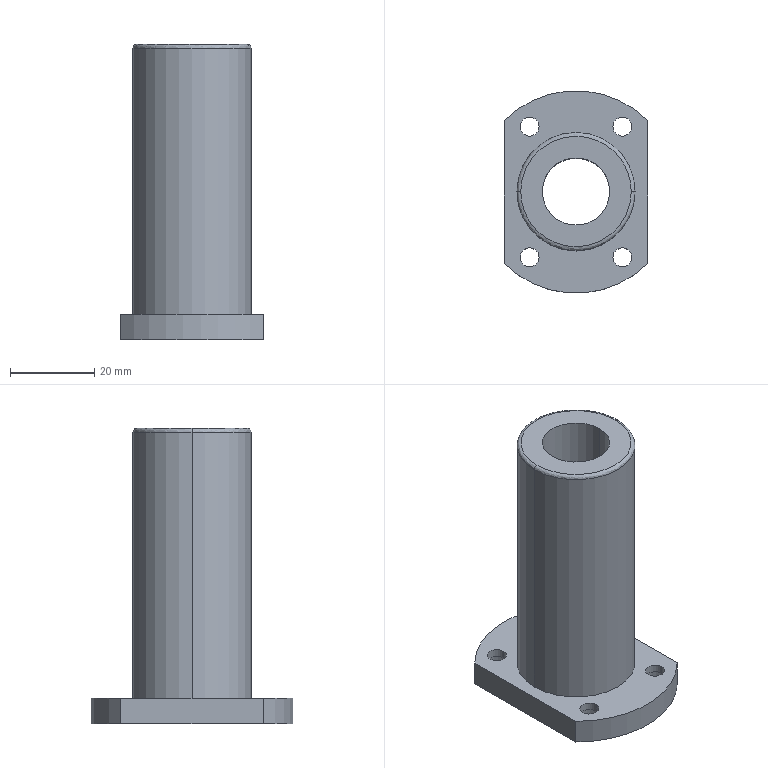Part | SolidWorks | features BaseBody 1 | 1 solid | 33 faces | box 34 x 48 x 70 mm | volume 33372 mm3 | cylinder 22 | plane 9 | spline 2 | commonest cylinder face diameters 4.5 x8 7.5 x8 16 x2 28 x2 48 x2
STEP:
#1=CARTESIAN_POINT('',(14.,0.,69.1));
#2=VERTEX_POINT('',#1);
#3=CARTESIAN_POINT('',(-14.,0.,69.1));
#4=VERTEX_POINT('',#3);
#5=CARTESIAN_POINT('',(0.,0.,69.1));
#6=DIRECTION('',(0.,0.,-1.));
#7=DIRECTION('',(-1.,0.,0.));
#8=AXIS2_PLACEMENT_3D('',#5,#6,#7);
#9=CIRCLE('',#8,14.);
#10=EDGE_CURVE('',#2,#4,#9,.T.);
#11=ORIENTED_EDGE('',*,*,#10,.F.);
#12=CARTESIAN_POINT('',(13.1,0.,70.));
#13=VERTEX_POINT('',#12);
#14=CARTESIAN_POINT('',(13.1,0.,69.1));
#15=DIRECTION('',(0.,-1.,0.));
#16=DIRECTION('',(1.,0.,0.));
#17=AXIS2_PLACEMENT_3D('',#14,#15,#16);
#18=CIRCLE('',#17,0.9);
#19=EDGE_CURVE('',#2,#13,#18,.T.);
#20=ORIENTED_EDGE('',*,*,#19,.T.);
#21=CARTESIAN_POINT('',(-13.1,0.,70.));
#22=VERTEX_POINT('',#21);
#23=CARTESIAN_POINT('',(13.1,0.,70.));
#24=CARTESIAN_POINT('',(13.1,-26.2,70.));
#25=CARTESIAN_POINT('',(-13.1,-26.2,70.));
#26=CARTESIAN_POINT('',(-13.1,0.,70.));
#27=(BOUNDED_CURVE()B_SPLINE_CURVE(3,(#23,#24,#25,#26),.UNSPECIFIED.,.F.,.F.)B_SPLINE_CURVE_WITH_KNOTS((4,4),(0.5,1.),.UNSPECIFIED.)CURVE()GEOMETRIC_REPRESENTATION_ITEM()RATIONAL_B_SPLINE_CURVE((1.,0.3333,0.3333,1.))REPRESENTATION_ITEM(''));
#28=EDGE_CURVE('',#13,#22,#27,.T.);
#29=ORIENTED_EDGE('',*,*,#28,.T.);
#30=CARTESIAN_POINT('',(-13.1,0.,69.1));
#31=DIRECTION('',(0.,1.,0.));
#32=DIRECTION('',(-1.,0.,0.));
#33=AXIS2_PLACEMENT_3D('',#30,#31,#32);
#34=CIRCLE('',#33,0.9);
#35=EDGE_CURVE('',#4,#22,#34,.T.);
#36=ORIENTED_EDGE('',*,*,#35,.F.);
#37=EDGE_LOOP('',(#11,#20,#29,#36));
#38=FACE_OUTER_BOUND('',#37,.T.);
#39=CARTESIAN_POINT('',(14.,0.,69.1));
#40=CARTESIAN_POINT('',(14.,-28.,69.1));
#41=CARTESIAN_POINT('',(-14.,-28.,69.1));
#42=CARTESIAN_POINT('',(-14.,0.,69.1));
#43=CARTESIAN_POINT('',(14.,0.,69.627));
#44=CARTESIAN_POINT('',(14.,-28.,69.627));
#45=CARTESIAN_POINT('',(-14.,-28.,69.627));
#46=CARTESIAN_POINT('',(-14.,0.,69.627));
#47=CARTESIAN_POINT('',(13.627,0.,70.));
#48=CARTESIAN_POINT('',(13.627,-27.254,70.));
#49=CARTESIAN_POINT('',(-13.627,-27.254,70.));
#50=CARTESIAN_POINT('',(-13.627,0.,70.));
#51=CARTESIAN_POINT('',(13.1,0.,70.));
#52=CARTESIAN_POINT('',(13.1,-26.2,70.));
#53=CARTESIAN_POINT('',(-13.1,-26.2,70.));
#54=CARTESIAN_POINT('',(-13.1,0.,70.));
#55=(BOUNDED_SURFACE()B_SPLINE_SURFACE(3,3,((#39,#40,#41,#42),(#43,#44,#45,#46),(#47,#48,#49,#50),(#51,#52,#53,#54)),.UNSPECIFIED.,.F.,.F.,.F.)B_SPLINE_SURFACE_WITH_KNOTS((4,4),(4,4),(0.,1.),(0.,1.),.UNSPECIFIED.)GEOMETRIC_REPRESENTATION_ITEM()RATIONAL_B_SPLINE_SURFACE(((1.,0.3333,0.3333,1.),(0.8047,0.2682,0.2682,0.8047),(0.8047,0.2682,0.2682,0.8047),(1.,0.3333,0.3333,1.)))REPRESENTATION_ITEM('')SURFACE());
#56=ADVANCED_FACE('',(#38),#55,.T.);
#57=CARTESIAN_POINT('',(0.,0.,69.1));
#58=DIRECTION('',(0.,0.,-1.));
#59=DIRECTION('',(-1.,0.,0.));
#60=AXIS2_PLACEMENT_3D('',#57,#58,#59);
#61=CIRCLE('',#60,14.);
#62=EDGE_CURVE('',#4,#2,#61,.T.);
#63=ORIENTED_EDGE('',*,*,#62,.T.);
#64=CARTESIAN_POINT('',(14.,0.,6.));
#65=VERTEX_POINT('',#64);
#66=CARTESIAN_POINT('',(14.,0.,0.));
#67=DIRECTION('',(0.,0.,-1.));
#68=VECTOR('',#67,1000.);
#69=LINE('',#66,#68);
#70=EDGE_CURVE('',#2,#65,#69,.T.);
#71=ORIENTED_EDGE('',*,*,#70,.T.);
#72=CARTESIAN_POINT('',(-14.,0.,6.));
#73=VERTEX_POINT('',#72);
#74=CARTESIAN_POINT('',(0.,0.,6.));
#75=DIRECTION('',(0.,0.,1.));
#76=DIRECTION('',(-1.,0.,0.));
#77=AXIS2_PLACEMENT_3D('',#74,#75,#76);
#78=CIRCLE('',#77,14.);
#79=EDGE_CURVE('',#65,#73,#78,.T.);
#80=ORIENTED_EDGE('',*,*,#79,.T.);
#81=CARTESIAN_POINT('',(-14.,0.,0.));
#82=DIRECTION('',(0.,0.,-1.));
#83=VECTOR('',#82,1000.);
#84=LINE('',#81,#83);
#85=EDGE_CURVE('',#4,#73,#84,.T.);
#86=ORIENTED_EDGE('',*,*,#85,.F.);
#87=EDGE_LOOP('',(#63,#71,#80,#86));
#88=FACE_OUTER_BOUND('',#87,.T.);
#89=CARTESIAN_POINT('',(0.,0.,0.));
#90=DIRECTION('',(0.,0.,-1.));
#91=DIRECTION('',(-1.,0.,0.));
#92=AXIS2_PLACEMENT_3D('',#89,#90,#91);
#93=CYLINDRICAL_SURFACE('',#92,14.);
#94=ADVANCED_FACE('',(#88),#93,.T.);
#95=CARTESIAN_POINT('',(-8.75,15.5,6.));
#96=VERTEX_POINT('',#95);
#97=CARTESIAN_POINT('',(-13.25,15.5,6.));
#98=VERTEX_POINT('',#97);
#99=CARTESIAN_POINT('',(-11.,15.5,6.));
#100=DIRECTION('',(0.,0.,-1.));
#101=DIRECTION('',(-1.,0.,0.));
#102=AXIS2_PLACEMENT_3D('',#99,#100,#101);
#103=CIRCLE('',#102,2.25);
#104=EDGE_CURVE('',#96,#98,#103,.T.);
#105=ORIENTED_EDGE('',*,*,#104,.F.);
#106=CARTESIAN_POINT('',(-8.75,15.5,4.1));
#107=VERTEX_POINT('',#106);
#108=CARTESIAN_POINT('',(-8.75,15.5,0.));
#109=DIRECTION('',(0.,0.,-1.));
#110=VECTOR('',#109,1000.);
#111=LINE('',#108,#110);
#112=EDGE_CURVE('',#96,#107,#111,.T.);
#113=ORIENTED_EDGE('',*,*,#112,.T.);
#114=CARTESIAN_POINT('',(-13.25,15.5,4.1));
#115=VERTEX_POINT('',#114);
#116=CARTESIAN_POINT('',(-11.,15.5,4.1));
#117=DIRECTION('',(0.,0.,1.));
#118=DIRECTION('',(-1.,0.,0.));
#119=AXIS2_PLACEMENT_3D('',#116,#117,#118);
#120=CIRCLE('',#119,2.25);
#121=EDGE_CURVE('',#115,#107,#120,.T.);
#122=ORIENTED_EDGE('',*,*,#121,.F.);
#123=CARTESIAN_POINT('',(-13.25,15.5,0.));
#124=DIRECTION('',(0.,0.,-1.));
#125=VECTOR('',#124,1000.);
#126=LINE('',#123,#125);
#127=EDGE_CURVE('',#98,#115,#126,.T.);
#128=ORIENTED_EDGE('',*,*,#127,.F.);
#129=EDGE_LOOP('',(#105,#113,#122,#128));
#130=FACE_OUTER_BOUND('',#129,.T.);
#131=CARTESIAN_POINT('',(-11.,15.5,0.));
#132=DIRECTION('',(0.,0.,-1.));
#133=DIRECTION('',(-1.,0.,0.));
#134=AXIS2_PLACEMENT_3D('',#131,#132,#133);
#135=CYLINDRICAL_SURFACE('',#134,2.25);
#136=ADVANCED_FACE('',(#130),#135,.F.);
#137=CARTESIAN_POINT('',(-13.25,-15.5,4.1));
#138=VERTEX_POINT('',#137);
#139=CARTESIAN_POINT('',(-8.75,-15.5,4.1));
#140=VERTEX_POINT('',#139);
#141=CARTESIAN_POINT('',(-11.,-15.5,4.1));
#142=DIRECTION('',(0.,0.,1.));
#143=DIRECTION('',(1.,0.,0.));
#144=AXIS2_PLACEMENT_3D('',#141,#142,#143);
#145=CIRCLE('',#144,2.25);
#146=EDGE_CURVE('',#138,#140,#145,.T.);
#147=ORIENTED_EDGE('',*,*,#146,.F.);
#148=CARTESIAN_POINT('',(-13.25,-15.5,6.));
#149=VERTEX_POINT('',#148);
#150=CARTESIAN_POINT('',(-13.25,-15.5,6.));
#151=DIRECTION('',(0.,0.,1.));
#152=VECTOR('',#151,1000.);
#153=LINE('',#150,#152);
#154=EDGE_CURVE('',#138,#149,#153,.T.);
#155=ORIENTED_EDGE('',*,*,#154,.T.);
#156=CARTESIAN_POINT('',(-8.75,-15.5,6.));
#157=VERTEX_POINT('',#156);
#158=CARTESIAN_POINT('',(-11.,-15.5,6.));
#159=DIRECTION('',(0.,0.,-1.));
#160=DIRECTION('',(1.,0.,0.));
#161=AXIS2_PLACEMENT_3D('',#158,#159,#160);
#162=CIRCLE('',#161,2.25);
#163=EDGE_CURVE('',#157,#149,#162,.T.);
#164=ORIENTED_EDGE('',*,*,#163,.F.);
#165=CARTESIAN_POINT('',(-8.75,-15.5,6.));
#166=DIRECTION('',(0.,0.,1.));
#167=VECTOR('',#166,1000.);
#168=LINE('',#165,#167);
#169=EDGE_CURVE('',#140,#157,#168,.T.);
#170=ORIENTED_EDGE('',*,*,#169,.F.);
#171=EDGE_LOOP('',(#147,#155,#164,#170));
#172=FACE_OUTER_BOUND('',#171,.T.);
#173=CARTESIAN_POINT('',(-11.,-15.5,6.));
#174=DIRECTION('',(0.,0.,1.));
#175=DIRECTION('',(1.,0.,0.));
#176=AXIS2_PLACEMENT_3D('',#173,#174,#175);
#177=CYLINDRICAL_SURFACE('',#176,2.25);
#178=ADVANCED_FACE('',(#172),#177,.F.);
#179=CARTESIAN_POINT('',(13.25,15.5,6.));
#180=VERTEX_POINT('',#179);
#181=CARTESIAN_POINT('',(8.75,15.5,6.));
#182=VERTEX_POINT('',#181);
#183=CARTESIAN_POINT('',(11.,15.5,6.));
#184=DIRECTION('',(0.,0.,-1.));
#185=DIRECTION('',(-1.,0.,0.));
#186=AXIS2_PLACEMENT_3D('',#183,#184,#185);
#187=CIRCLE('',#186,2.25);
#188=EDGE_CURVE('',#180,#182,#187,.T.);
#189=ORIENTED_EDGE('',*,*,#188,.F.);
#190=CARTESIAN_POINT('',(13.25,15.5,4.1));
#191=VERTEX_POINT('',#190);
#192=CARTESIAN_POINT('',(13.25,15.5,0.));
#193=DIRECTION('',(0.,0.,-1.));
#194=VECTOR('',#193,1000.);
#195=LINE('',#192,#194);
#196=EDGE_CURVE('',#180,#191,#195,.T.);
#197=ORIENTED_EDGE('',*,*,#196,.T.);
#198=CARTESIAN_POINT('',(8.75,15.5,4.1));
#199=VERTEX_POINT('',#198);
#200=CARTESIAN_POINT('',(11.,15.5,4.1));
#201=DIRECTION('',(0.,0.,1.));
#202=DIRECTION('',(-1.,0.,0.));
#203=AXIS2_PLACEMENT_3D('',#200,#201,#202);
#204=CIRCLE('',#203,2.25);
#205=EDGE_CURVE('',#199,#191,#204,.T.);
#206=ORIENTED_EDGE('',*,*,#205,.F.);
#207=CARTESIAN_POINT('',(8.75,15.5,0.));
#208=DIRECTION('',(0.,0.,-1.));
#209=VECTOR('',#208,1000.);
#210=LINE('',#207,#209);
#211=EDGE_CURVE('',#182,#199,#210,.T.);
#212=ORIENTED_EDGE('',*,*,#211,.F.);
#213=EDGE_LOOP('',(#189,#197,#206,#212));
#214=FACE_OUTER_BOUND('',#213,.T.);
#215=CARTESIAN_POINT('',(11.,15.5,0.));
#216=DIRECTION('',(0.,0.,-1.));
#217=DIRECTION('',(-1.,0.,0.));
#218=AXIS2_PLACEMENT_3D('',#215,#216,#217);
#219=CYLINDRICAL_SURFACE('',#218,2.25);
#220=ADVANCED_FACE('',(#214),#219,.F.);
#221=CARTESIAN_POINT('',(8.75,-15.5,4.1));
#222=VERTEX_POINT('',#221);
#223=CARTESIAN_POINT('',(13.25,-15.5,4.1));
#224=VERTEX_POINT('',#223);
#225=CARTESIAN_POINT('',(11.,-15.5,4.1));
#226=DIRECTION('',(0.,0.,1.));
#227=DIRECTION('',(1.,0.,0.));
#228=AXIS2_PLACEMENT_3D('',#225,#226,#227);
#229=CIRCLE('',#228,2.25);
#230=EDGE_CURVE('',#222,#224,#229,.T.);
#231=ORIENTED_EDGE('',*,*,#230,.F.);
#232=CARTESIAN_POINT('',(8.75,-15.5,6.));
#233=VERTEX_POINT('',#232);
#234=CARTESIAN_POINT('',(8.75,-15.5,6.));
#235=DIRECTION('',(0.,0.,1.));
#236=VECTOR('',#235,1000.);
#237=LINE('',#234,#236);
#238=EDGE_CURVE('',#222,#233,#237,.T.);
#239=ORIENTED_EDGE('',*,*,#238,.T.);
#240=CARTESIAN_POINT('',(13.25,-15.5,6.));
#241=VERTEX_POINT('',#240);
#242=CARTESIAN_POINT('',(11.,-15.5,6.));
#243=DIRECTION('',(0.,0.,-1.));
#244=DIRECTION('',(1.,0.,0.));
#245=AXIS2_PLACEMENT_3D('',#242,#243,#244);
#246=CIRCLE('',#245,2.25);
#247=EDGE_CURVE('',#241,#233,#246,.T.);
#248=ORIENTED_EDGE('',*,*,#247,.F.);
#249=CARTESIAN_POINT('',(13.25,-15.5,6.));
#250=DIRECTION('',(0.,0.,1.));
#251=VECTOR('',#250,1000.);
#252=LINE('',#249,#251);
#253=EDGE_CURVE('',#224,#241,#252,.T.);
#254=ORIENTED_EDGE('',*,*,#253,.F.);
#255=EDGE_LOOP('',(#231,#239,#248,#254));
#256=FACE_OUTER_BOUND('',#255,.T.);
#257=CARTESIAN_POINT('',(11.,-15.5,6.));
#258=DIRECTION('',(0.,0.,1.));
#259=DIRECTION('',(1.,0.,0.));
#260=AXIS2_PLACEMENT_3D('',#257,#258,#259);
#261=CYLINDRICAL_SURFACE('',#260,2.25);
#262=ADVANCED_FACE('',(#256),#261,.F.);
#263=CARTESIAN_POINT('',(8.,0.,70.));
#264=VERTEX_POINT('',#263);
#265=CARTESIAN_POINT('',(-8.,0.,70.));
#266=VERTEX_POINT('',#265);
#267=CARTESIAN_POINT('',(0.,0.,70.));
#268=DIRECTION('',(0.,0.,-1.));
#269=DIRECTION('',(-1.,0.,0.));
#270=AXIS2_PLACEMENT_3D('',#267,#268,#269);
#271=CIRCLE('',#270,8.);
#272=EDGE_CURVE('',#264,#266,#271,.T.);
#273=ORIENTED_EDGE('',*,*,#272,.F.);
#274=CARTESIAN_POINT('',(8.,0.,0.));
#275=VERTEX_POINT('',#274);
#276=CARTESIAN_POINT('',(8.,0.,0.));
#277=DIRECTION('',(0.,0.,-1.));
#278=VECTOR('',#277,1000.);
#279=LINE('',#276,#278);
#280=EDGE_CURVE('',#264,#275,#279,.T.);
#281=ORIENTED_EDGE('',*,*,#280,.T.);
#282=CARTESIAN_POINT('',(-8.,0.,0.));
#283=VERTEX_POINT('',#282);
#284=CARTESIAN_POINT('',(0.,0.,0.));
#285=DIRECTION('',(0.,0.,1.));
#286=DIRECTION('',(-1.,0.,0.));
#287=AXIS2_PLACEMENT_3D('',#284,#285,#286);
#288=CIRCLE('',#287,8.);
#289=EDGE_CURVE('',#283,#275,#288,.T.);
#290=ORIENTED_EDGE('',*,*,#289,.F.);
#291=CARTESIAN_POINT('',(-8.,0.,0.));
#292=DIRECTION('',(0.,0.,-1.));
#293=VECTOR('',#292,1000.);
#294=LINE('',#291,#293);
#295=EDGE_CURVE('',#266,#283,#294,.T.);
#296=ORIENTED_EDGE('',*,*,#295,.F.);
#297=EDGE_LOOP('',(#273,#281,#290,#296));
#298=FACE_OUTER_BOUND('',#297,.T.);
#299=CARTESIAN_POINT('',(0.,0.,0.));
#300=DIRECTION('',(0.,0.,-1.));
#301=DIRECTION('',(-1.,0.,0.));
#302=AXIS2_PLACEMENT_3D('',#299,#300,#301);
#303=CYLINDRICAL_SURFACE('',#302,8.);
#304=ADVANCED_FACE('',(#298),#303,.F.);
#305=CARTESIAN_POINT('',(-7.25,15.5,4.1));
#306=VERTEX_POINT('',#305);
#307=CARTESIAN_POINT('',(-14.75,15.5,4.1));
#308=VERTEX_POINT('',#307);
#309=CARTESIAN_POINT('',(-11.,15.5,4.1));
#310=DIRECTION('',(0.,0.,-1.));
#311=DIRECTION('',(-1.,0.,0.));
#312=AXIS2_PLACEMENT_3D('',#309,#310,#311);
#313=CIRCLE('',#312,3.75);
#314=EDGE_CURVE('',#306,#308,#313,.T.);
#315=ORIENTED_EDGE('',*,*,#314,.F.);
#316=CARTESIAN_POINT('',(-7.25,15.5,0.));
#317=VERTEX_POINT('',#316);
#318=CARTESIAN_POINT('',(-7.25,15.5,0.));
#319=DIRECTION('',(0.,0.,-1.));
#320=VECTOR('',#319,1000.);
#321=LINE('',#318,#320);
#322=EDGE_CURVE('',#306,#317,#321,.T.);
#323=ORIENTED_EDGE('',*,*,#322,.T.);
#324=CARTESIAN_POINT('',(-14.75,15.5,0.));
#325=VERTEX_POINT('',#324);
#326=CARTESIAN_POINT('',(-11.,15.5,0.));
#327=DIRECTION('',(0.,0.,1.));
#328=DIRECTION('',(-1.,0.,0.));
#329=AXIS2_PLACEMENT_3D('',#326,#327,#328);
#330=CIRCLE('',#329,3.75);
#331=EDGE_CURVE('',#325,#317,#330,.T.);
#332=ORIENTED_EDGE('',*,*,#331,.F.);
#333=CARTESIAN_POINT('',(-14.75,15.5,0.));
#334=DIRECTION('',(0.,0.,-1.));
#335=VECTOR('',#334,1000.);
#336=LINE('',#333,#335);
#337=EDGE_CURVE('',#308,#325,#336,.T.);
#338=ORIENTED_EDGE('',*,*,#337,.F.);
#339=EDGE_LOOP('',(#315,#323,#332,#338));
#340=FACE_OUTER_BOUND('',#339,.T.);
#341=CARTESIAN_POINT('',(-11.,15.5,0.));
#342=DIRECTION('',(0.,0.,-1.));
#343=DIRECTION('',(-1.,0.,0.));
#344=AXIS2_PLACEMENT_3D('',#341,#342,#343);
#345=CYLINDRICAL_SURFACE('',#344,3.75);
#346=ADVANCED_FACE('',(#340),#345,.F.);
#347=CARTESIAN_POINT('',(-14.75,-15.5,0.));
#348=VERTEX_POINT('',#347);
#349=CARTESIAN_POINT('',(-7.25,-15.5,0.));
#350=VERTEX_POINT('',#349);
#351=CARTESIAN_POINT('',(-11.,-15.5,0.));
#352=DIRECTION('',(0.,0.,1.));
#353=DIRECTION('',(1.,0.,0.));
#354=AXIS2_PLACEMENT_3D('',#351,#352,#353);
#355=CIRCLE('',#354,3.75);
#356=EDGE_CURVE('',#348,#350,#355,.T.);
#357=ORIENTED_EDGE('',*,*,#356,.F.);
#358=CARTESIAN_POINT('',(-14.75,-15.5,4.1));
#359=VERTEX_POINT('',#358);
#360=CARTESIAN_POINT('',(-14.75,-15.5,6.));
#361=DIRECTION('',(0.,0.,1.));
#362=VECTOR('',#361,1000.);
#363=LINE('',#360,#362);
#364=EDGE_CURVE('',#348,#359,#363,.T.);
#365=ORIENTED_EDGE('',*,*,#364,.T.);
#366=CARTESIAN_POINT('',(-7.25,-15.5,4.1));
#367=VERTEX_POINT('',#366);
#368=CARTESIAN_POINT('',(-11.,-15.5,4.1));
#369=DIRECTION('',(0.,0.,-1.));
#370=DIRECTION('',(1.,0.,0.));
#371=AXIS2_PLACEMENT_3D('',#368,#369,#370);
#372=CIRCLE('',#371,3.75);
#373=EDGE_CURVE('',#367,#359,#372,.T.);
#374=ORIENTED_EDGE('',*,*,#373,.F.);
#375=CARTESIAN_POINT('',(-7.25,-15.5,6.));
#376=DIRECTION('',(0.,0.,1.));
#377=VECTOR('',#376,1000.);
#378=LINE('',#375,#377);
#379=EDGE_CURVE('',#350,#367,#378,.T.);
#380=ORIENTED_EDGE('',*,*,#379,.F.);
#381=EDGE_LOOP('',(#357,#365,#374,#380));
#382=FACE_OUTER_BOUND('',#381,.T.);
#383=CARTESIAN_POINT('',(-11.,-15.5,6.));
#384=DIRECTION('',(0.,0.,1.));
#385=DIRECTION('',(1.,0.,0.));
#386=AXIS2_PLACEMENT_3D('',#383,#384,#385);
#387=CYLINDRICAL_SURFACE('',#386,3.75);
#388=ADVANCED_FACE('',(#382),#387,.F.);
#389=CARTESIAN_POINT('',(14.75,15.5,4.1));
#390=VERTEX_POINT('',#389);
#391=CARTESIAN_POINT('',(7.25,15.5,4.1));
#392=VERTEX_POINT('',#391);
#393=CARTESIAN_POINT('',(11.,15.5,4.1));
#394=DIRECTION('',(0.,0.,-1.));
#395=DIRECTION('',(-1.,0.,0.));
#396=AXIS2_PLACEMENT_3D('',#393,#394,#395);
#397=CIRCLE('',#396,3.75);
#398=EDGE_CURVE('',#390,#392,#397,.T.);
#399=ORIENTED_EDGE('',*,*,#398,.F.);
#400=CARTESIAN_POINT('',(14.75,15.5,0.));
#401=VERTEX_POINT('',#400);
#402=CARTESIAN_POINT('',(14.75,15.5,0.));
#403=DIRECTION('',(0.,0.,-1.));
#404=VECTOR('',#403,1000.);
#405=LINE('',#402,#404);
#406=EDGE_CURVE('',#390,#401,#405,.T.);
#407=ORIENTED_EDGE('',*,*,#406,.T.);
#408=CARTESIAN_POINT('',(7.25,15.5,0.));
#409=VERTEX_POINT('',#408);
#410=CARTESIAN_POINT('',(11.,15.5,0.));
#411=DIRECTION('',(0.,0.,1.));
#412=DIRECTION('',(-1.,0.,0.));
#413=AXIS2_PLACEMENT_3D('',#410,#411,#412);
#414=CIRCLE('',#413,3.75);
#415=EDGE_CURVE('',#409,#401,#414,.T.);
#416=ORIENTED_EDGE('',*,*,#415,.F.);
#417=CARTESIAN_POINT('',(7.25,15.5,0.));
#418=DIRECTION('',(0.,0.,-1.));
#419=VECTOR('',#418,1000.);
#420=LINE('',#417,#419);
#421=EDGE_CURVE('',#392,#409,#420,.T.);
#422=ORIENTED_EDGE('',*,*,#421,.F.);
#423=EDGE_LOOP('',(#399,#407,#416,#422));
#424=FACE_OUTER_BOUND('',#423,.T.);
#425=CARTESIAN_POINT('',(11.,15.5,0.));
#426=DIRECTION('',(0.,0.,-1.));
#427=DIRECTION('',(-1.,0.,0.));
#428=AXIS2_PLACEMENT_3D('',#425,#426,#427);
#429=CYLINDRICAL_SURFACE('',#428,3.75);
#430=ADVANCED_FACE('',(#424),#429,.F.);
#431=CARTESIAN_POINT('',(7.25,-15.5,0.));
#432=VERTEX_POINT('',#431);
#433=CARTESIAN_POINT('',(14.75,-15.5,0.));
#434=VERTEX_POINT('',#433);
#435=CARTESIAN_POINT('',(11.,-15.5,0.));
#436=DIRECTION('',(0.,0.,1.));
#437=DIRECTION('',(1.,0.,0.));
#438=AXIS2_PLACEMENT_3D('',#435,#436,#437);
#439=CIRCLE('',#438,3.75);
#440=EDGE_CURVE('',#432,#434,#439,.T.);
#441=ORIENTED_EDGE('',*,*,#440,.F.);
#442=CARTESIAN_POINT('',(7.25,-15.5,4.1));
#443=VERTEX_POINT('',#442);
#444=CARTESIAN_POINT('',(7.25,-15.5,6.));
#445=DIRECTION('',(0.,0.,1.));
#446=VECTOR('',#445,1000.);
#447=LINE('',#444,#446);
#448=EDGE_CURVE('',#432,#443,#447,.T.);
#449=ORIENTED_EDGE('',*,*,#448,.T.);
#450=CARTESIAN_POINT('',(14.75,-15.5,4.1));
#451=VERTEX_POINT('',#450);
#452=CARTESIAN_POINT('',(11.,-15.5,4.1));
#453=DIRECTION('',(0.,0.,-1.));
#454=DIRECTION('',(1.,0.,0.));
#455=AXIS2_PLACEMENT_3D('',#452,#453,#454);
#456=CIRCLE('',#455,3.75);
#457=EDGE_CURVE('',#451,#443,#456,.T.);
#458=ORIENTED_EDGE('',*,*,#457,.F.);
#459=CARTESIAN_POINT('',(14.75,-15.5,6.));
#460=DIRECTION('',(0.,0.,1.));
#461=VECTOR('',#460,1000.);
#462=LINE('',#459,#461);
#463=EDGE_CURVE('',#434,#451,#462,.T.);
#464=ORIENTED_EDGE('',*,*,#463,.F.);
#465=EDGE_LOOP('',(#441,#449,#458,#464));
#466=FACE_OUTER_BOUND('',#465,.T.);
#467=CARTESIAN_POINT('',(11.,-15.5,6.));
#468=DIRECTION('',(0.,0.,1.));
#469=DIRECTION('',(1.,0.,0.));
#470=AXIS2_PLACEMENT_3D('',#467,#468,#469);
#471=CYLINDRICAL_SURFACE('',#470,3.75);
#472=ADVANCED_FACE('',(#466),#471,.F.);
#473=ORIENTED_EDGE('',*,*,#70,.F.);
#474=ORIENTED_EDGE('',*,*,#10,.T.);
#475=ORIENTED_EDGE('',*,*,#85,.T.);
#476=CARTESIAN_POINT('',(0.,0.,6.));
#477=DIRECTION('',(0.,0.,1.));
#478=DIRECTION('',(-1.,0.,0.));
#479=AXIS2_PLACEMENT_3D('',#476,#477,#478);
#480=CIRCLE('',#479,14.);
#481=EDGE_CURVE('',#73,#65,#480,.T.);
#482=ORIENTED_EDGE('',*,*,#481,.T.);
#483=EDGE_LOOP('',(#473,#474,#475,#482));
#484=FACE_OUTER_BOUND('',#483,.T.);
#485=CARTESIAN_POINT('',(0.,0.,0.));
#486=DIRECTION('',(0.,0.,-1.));
#487=DIRECTION('',(-1.,0.,0.));
#488=AXIS2_PLACEMENT_3D('',#485,#486,#487);
#489=CYLINDRICAL_SURFACE('',#488,14.);
#490=ADVANCED_FACE('',(#484),#489,.T.);
#491=CARTESIAN_POINT('',(-17.,-16.941,6.));
#492=VERTEX_POINT('',#491);
#493=CARTESIAN_POINT('',(17.,-16.941,6.));
#494=VERTEX_POINT('',#493);
#495=CARTESIAN_POINT('',(0.,0.,6.));
#496=DIRECTION('',(0.,0.,1.));
#497=DIRECTION('',(-1.,0.,0.));
#498=AXIS2_PLACEMENT_3D('',#495,#496,#497);
#499=CIRCLE('',#498,24.);
#500=EDGE_CURVE('',#492,#494,#499,.T.);
#501=ORIENTED_EDGE('',*,*,#500,.T.);
#502=CARTESIAN_POINT('',(17.,16.941,6.));
#503=VERTEX_POINT('',#502);
#504=CARTESIAN_POINT('',(17.,0.,6.));
#505=DIRECTION('',(0.,1.,0.));
#506=VECTOR('',#505,1000.);
#507=LINE('',#504,#506);
#508=EDGE_CURVE('',#494,#503,#507,.T.);
#509=ORIENTED_EDGE('',*,*,#508,.T.);
#510=CARTESIAN_POINT('',(-17.,16.941,6.));
#511=VERTEX_POINT('',#510);
#512=CARTESIAN_POINT('',(0.,0.,6.));
#513=DIRECTION('',(0.,0.,1.));
#514=DIRECTION('',(-1.,0.,0.));
#515=AXIS2_PLACEMENT_3D('',#512,#513,#514);
#516=CIRCLE('',#515,24.);
#517=EDGE_CURVE('',#503,#511,#516,.T.);
#518=ORIENTED_EDGE('',*,*,#517,.T.);
#519=CARTESIAN_POINT('',(-17.,0.,6.));
#520=DIRECTION('',(0.,-1.,0.));
#521=VECTOR('',#520,1000.);
#522=LINE('',#519,#521);
#523=EDGE_CURVE('',#511,#492,#522,.T.);
#524=ORIENTED_EDGE('',*,*,#523,.T.);
#525=EDGE_LOOP('',(#501,#509,#518,#524));
#526=FACE_OUTER_BOUND('',#525,.T.);
#527=ORIENTED_EDGE('',*,*,#481,.F.);
#528=ORIENTED_EDGE('',*,*,#79,.F.);
#529=EDGE_LOOP('',(#527,#528));
#530=FACE_BOUND('',#529,.T.);
#531=CARTESIAN_POINT('',(-11.,15.5,6.));
#532=DIRECTION('',(0.,0.,-1.));
#533=DIRECTION('',(-1.,0.,0.));
#534=AXIS2_PLACEMENT_3D('',#531,#532,#533);
#535=CIRCLE('',#534,2.25);
#536=EDGE_CURVE('',#98,#96,#535,.T.);
#537=ORIENTED_EDGE('',*,*,#536,.T.);
#538=ORIENTED_EDGE('',*,*,#104,.T.);
#539=EDGE_LOOP('',(#537,#538));
#540=FACE_BOUND('',#539,.T.);
#541=ORIENTED_EDGE('',*,*,#163,.T.);
#542=CARTESIAN_POINT('',(-11.,-15.5,6.));
#543=DIRECTION('',(0.,0.,-1.));
#544=DIRECTION('',(1.,0.,0.));
#545=AXIS2_PLACEMENT_3D('',#542,#543,#544);
#546=CIRCLE('',#545,2.25);
#547=EDGE_CURVE('',#149,#157,#546,.T.);
#548=ORIENTED_EDGE('',*,*,#547,.T.);
#549=EDGE_LOOP('',(#541,#548));
#550=FACE_BOUND('',#549,.T.);
#551=CARTESIAN_POINT('',(11.,15.5,6.));
#552=DIRECTION('',(0.,0.,-1.));
#553=DIRECTION('',(-1.,0.,0.));
#554=AXIS2_PLACEMENT_3D('',#551,#552,#553);
#555=CIRCLE('',#554,2.25);
#556=EDGE_CURVE('',#182,#180,#555,.T.);
#557=ORIENTED_EDGE('',*,*,#556,.T.);
#558=ORIENTED_EDGE('',*,*,#188,.T.);
#559=EDGE_LOOP('',(#557,#558));
#560=FACE_BOUND('',#559,.T.);
#561=ORIENTED_EDGE('',*,*,#247,.T.);
#562=CARTESIAN_POINT('',(11.,-15.5,6.));
#563=DIRECTION('',(0.,0.,-1.));
#564=DIRECTION('',(1.,0.,0.));
#565=AXIS2_PLACEMENT_3D('',#562,#563,#564);
#566=CIRCLE('',#565,2.25);
#567=EDGE_CURVE('',#233,#241,#566,.T.);
#568=ORIENTED_EDGE('',*,*,#567,.T.);
#569=EDGE_LOOP('',(#561,#568));
#570=FACE_BOUND('',#569,.T.);
#571=CARTESIAN_POINT('',(0.,0.,6.));
#572=DIRECTION('',(0.,0.,1.));
#573=DIRECTION('',(1.,0.,0.));
#574=AXIS2_PLACEMENT_3D('',#571,#572,#573);
#575=PLANE('',#574);
#576=ADVANCED_FACE('',(#526,#530,#540,#550,#560,#570),#575,.T.);
#577=ORIENTED_EDGE('',*,*,#19,.F.);
#578=ORIENTED_EDGE('',*,*,#62,.F.);
#579=ORIENTED_EDGE('',*,*,#35,.T.);
#580=CARTESIAN_POINT('',(-13.1,0.,70.));
#581=CARTESIAN_POINT('',(-13.1,26.2,70.));
#582=CARTESIAN_POINT('',(13.1,26.2,70.));
#583=CARTESIAN_POINT('',(13.1,0.,70.));
#584=(BOUNDED_CURVE()B_SPLINE_CURVE(3,(#580,#581,#582,#583),.UNSPECIFIED.,.F.,.F.)B_SPLINE_CURVE_WITH_KNOTS((4,4),(0.,0.5),.UNSPECIFIED.)CURVE()GEOMETRIC_REPRESENTATION_ITEM()RATIONAL_B_SPLINE_CURVE((1.,0.3333,0.3333,1.))REPRESENTATION_ITEM(''));
#585=EDGE_CURVE('',#22,#13,#584,.T.);
#586=ORIENTED_EDGE('',*,*,#585,.T.);
#587=EDGE_LOOP('',(#577,#578,#579,#586));
#588=FACE_OUTER_BOUND('',#587,.T.);
#589=CARTESIAN_POINT('',(-14.,0.,69.1));
#590=CARTESIAN_POINT('',(-14.,28.,69.1));
#591=CARTESIAN_POINT('',(14.,28.,69.1));
#592=CARTESIAN_POINT('',(14.,0.,69.1));
#593=CARTESIAN_POINT('',(-14.,0.,69.627));
#594=CARTESIAN_POINT('',(-14.,28.,69.627));
#595=CARTESIAN_POINT('',(14.,28.,69.627));
#596=CARTESIAN_POINT('',(14.,0.,69.627));
#597=CARTESIAN_POINT('',(-13.627,0.,70.));
#598=CARTESIAN_POINT('',(-13.627,27.254,70.));
#599=CARTESIAN_POINT('',(13.627,27.254,70.));
#600=CARTESIAN_POINT('',(13.627,0.,70.));
#601=CARTESIAN_POINT('',(-13.1,0.,70.));
#602=CARTESIAN_POINT('',(-13.1,26.2,70.));
#603=CARTESIAN_POINT('',(13.1,26.2,70.));
#604=CARTESIAN_POINT('',(13.1,0.,70.));
#605=(BOUNDED_SURFACE()B_SPLINE_SURFACE(3,3,((#589,#590,#591,#592),(#593,#594,#595,#596),(#597,#598,#599,#600),(#601,#602,#603,#604)),.UNSPECIFIED.,.F.,.F.,.F.)B_SPLINE_SURFACE_WITH_KNOTS((4,4),(4,4),(0.,1.),(0.,1.),.UNSPECIFIED.)GEOMETRIC_REPRESENTATION_ITEM()RATIONAL_B_SPLINE_SURFACE(((1.,0.3333,0.3333,1.),(0.8047,0.2682,0.2682,0.8047),(0.8047,0.2682,0.2682,0.8047),(1.,0.3333,0.3333,1.)))REPRESENTATION_ITEM('')SURFACE());
#606=ADVANCED_FACE('',(#588),#605,.T.);
#607=CARTESIAN_POINT('',(17.,16.941,0.));
#608=VERTEX_POINT('',#607);
#609=CARTESIAN_POINT('',(17.,16.941,6.));
#610=DIRECTION('',(0.,0.,-1.));
#611=VECTOR('',#610,1000.);
#612=LINE('',#609,#611);
#613=EDGE_CURVE('',#503,#608,#612,.T.);
#614=ORIENTED_EDGE('',*,*,#613,.F.);
#615=ORIENTED_EDGE('',*,*,#508,.F.);
#616=CARTESIAN_POINT('',(17.,-16.941,0.));
#617=VERTEX_POINT('',#616);
#618=CARTESIAN_POINT('',(17.,-16.941,6.));
#619=DIRECTION('',(0.,0.,1.));
#620=VECTOR('',#619,1000.);
#621=LINE('',#618,#620);
#622=EDGE_CURVE('',#617,#494,#621,.T.);
#623=ORIENTED_EDGE('',*,*,#622,.F.);
#624=CARTESIAN_POINT('',(17.,-16.941,0.));
#625=DIRECTION('',(0.,-1.,0.));
#626=VECTOR('',#625,1000.);
#627=LINE('',#624,#626);
#628=EDGE_CURVE('',#608,#617,#627,.T.);
#629=ORIENTED_EDGE('',*,*,#628,.F.);
#630=EDGE_LOOP('',(#614,#615,#623,#629));
#631=FACE_OUTER_BOUND('',#630,.T.);
#632=CARTESIAN_POINT('',(17.,-16.941,6.));
#633=DIRECTION('',(-1.,0.,0.));
#634=DIRECTION('',(0.,0.,1.));
#635=AXIS2_PLACEMENT_3D('',#632,#633,#634);
#636=PLANE('',#635);
#637=ADVANCED_FACE('',(#631),#636,.F.);
#638=ORIENTED_EDGE('',*,*,#500,.F.);
#639=CARTESIAN_POINT('',(-17.,-16.941,0.));
#640=VERTEX_POINT('',#639);
#641=CARTESIAN_POINT('',(-17.,-16.941,6.));
#642=DIRECTION('',(0.,0.,-1.));
#643=VECTOR('',#642,1000.);
#644=LINE('',#641,#643);
#645=EDGE_CURVE('',#492,#640,#644,.T.);
#646=ORIENTED_EDGE('',*,*,#645,.T.);
#647=CARTESIAN_POINT('',(0.,0.,0.));
#648=DIRECTION('',(0.,0.,1.));
#649=DIRECTION('',(-1.,0.,0.));
#650=AXIS2_PLACEMENT_3D('',#647,#648,#649);
#651=CIRCLE('',#650,24.);
#652=EDGE_CURVE('',#640,#617,#651,.T.);
#653=ORIENTED_EDGE('',*,*,#652,.T.);
#654=ORIENTED_EDGE('',*,*,#622,.T.);
#655=EDGE_LOOP('',(#638,#646,#653,#654));
#656=FACE_OUTER_BOUND('',#655,.T.);
#657=CARTESIAN_POINT('',(0.,0.,6.));
#658=DIRECTION('',(0.,0.,-1.));
#659=DIRECTION('',(-1.,0.,0.));
#660=AXIS2_PLACEMENT_3D('',#657,#658,#659);
#661=CYLINDRICAL_SURFACE('',#660,24.);
#662=ADVANCED_FACE('',(#656),#661,.T.);
#663=ORIENTED_EDGE('',*,*,#645,.F.);
#664=ORIENTED_EDGE('',*,*,#523,.F.);
#665=CARTESIAN_POINT('',(-17.,16.941,0.));
#666=VERTEX_POINT('',#665);
#667=CARTESIAN_POINT('',(-17.,16.941,6.));
#668=DIRECTION('',(0.,0.,1.));
#669=VECTOR('',#668,1000.);
#670=LINE('',#667,#669);
#671=EDGE_CURVE('',#666,#511,#670,.T.);
#672=ORIENTED_EDGE('',*,*,#671,.F.);
#673=CARTESIAN_POINT('',(-17.,16.941,0.));
#674=DIRECTION('',(0.,1.,0.));
#675=VECTOR('',#674,1000.);
#676=LINE('',#673,#675);
#677=EDGE_CURVE('',#640,#666,#676,.T.);
#678=ORIENTED_EDGE('',*,*,#677,.F.);
#679=EDGE_LOOP('',(#663,#664,#672,#678));
#680=FACE_OUTER_BOUND('',#679,.T.);
#681=CARTESIAN_POINT('',(-17.,16.941,6.));
#682=DIRECTION('',(1.,0.,0.));
#683=DIRECTION('',(0.,0.,-1.));
#684=AXIS2_PLACEMENT_3D('',#681,#682,#683);
#685=PLANE('',#684);
#686=ADVANCED_FACE('',(#680),#685,.F.);
#687=ORIENTED_EDGE('',*,*,#517,.F.);
#688=ORIENTED_EDGE('',*,*,#613,.T.);
#689=CARTESIAN_POINT('',(0.,0.,0.));
#690=DIRECTION('',(0.,0.,1.));
#691=DIRECTION('',(-1.,0.,0.));
#692=AXIS2_PLACEMENT_3D('',#689,#690,#691);
#693=CIRCLE('',#692,24.);
#694=EDGE_CURVE('',#608,#666,#693,.T.);
#695=ORIENTED_EDGE('',*,*,#694,.T.);
#696=ORIENTED_EDGE('',*,*,#671,.T.);
#697=EDGE_LOOP('',(#687,#688,#695,#696));
#698=FACE_OUTER_BOUND('',#697,.T.);
#699=CARTESIAN_POINT('',(0.,0.,6.));
#700=DIRECTION('',(0.,0.,-1.));
#701=DIRECTION('',(-1.,0.,0.));
#702=AXIS2_PLACEMENT_3D('',#699,#700,#701);
#703=CYLINDRICAL_SURFACE('',#702,24.);
#704=ADVANCED_FACE('',(#698),#703,.T.);
#705=ORIENTED_EDGE('',*,*,#112,.F.);
#706=ORIENTED_EDGE('',*,*,#536,.F.);
#707=ORIENTED_EDGE('',*,*,#127,.T.);
#708=CARTESIAN_POINT('',(-11.,15.5,4.1));
#709=DIRECTION('',(0.,0.,1.));
#710=DIRECTION('',(-1.,0.,0.));
#711=AXIS2_PLACEMENT_3D('',#708,#709,#710);
#712=CIRCLE('',#711,2.25);
#713=EDGE_CURVE('',#107,#115,#712,.T.);
#714=ORIENTED_EDGE('',*,*,#713,.F.);
#715=EDGE_LOOP('',(#705,#706,#707,#714));
#716=FACE_OUTER_BOUND('',#715,.T.);
#717=CARTESIAN_POINT('',(-11.,15.5,0.));
#718=DIRECTION('',(0.,0.,-1.));
#719=DIRECTION('',(-1.,0.,0.));
#720=AXIS2_PLACEMENT_3D('',#717,#718,#719);
#721=CYLINDRICAL_SURFACE('',#720,2.25);
#722=ADVANCED_FACE('',(#716),#721,.F.);
#723=ORIENTED_EDGE('',*,*,#154,.F.);
#724=CARTESIAN_POINT('',(-11.,-15.5,4.1));
#725=DIRECTION('',(0.,0.,1.));
#726=DIRECTION('',(1.,0.,0.));
#727=AXIS2_PLACEMENT_3D('',#724,#725,#726);
#728=CIRCLE('',#727,2.25);
#729=EDGE_CURVE('',#140,#138,#728,.T.);
#730=ORIENTED_EDGE('',*,*,#729,.F.);
#731=ORIENTED_EDGE('',*,*,#169,.T.);
#732=ORIENTED_EDGE('',*,*,#547,.F.);
#733=EDGE_LOOP('',(#723,#730,#731,#732));
#734=FACE_OUTER_BOUND('',#733,.T.);
#735=CARTESIAN_POINT('',(-11.,-15.5,6.));
#736=DIRECTION('',(0.,0.,1.));
#737=DIRECTION('',(1.,0.,0.));
#738=AXIS2_PLACEMENT_3D('',#735,#736,#737);
#739=CYLINDRICAL_SURFACE('',#738,2.25);
#740=ADVANCED_FACE('',(#734),#739,.F.);
#741=ORIENTED_EDGE('',*,*,#196,.F.);
#742=ORIENTED_EDGE('',*,*,#556,.F.);
#743=ORIENTED_EDGE('',*,*,#211,.T.);
#744=CARTESIAN_POINT('',(11.,15.5,4.1));
#745=DIRECTION('',(0.,0.,1.));
#746=DIRECTION('',(-1.,0.,0.));
#747=AXIS2_PLACEMENT_3D('',#744,#745,#746);
#748=CIRCLE('',#747,2.25);
#749=EDGE_CURVE('',#191,#199,#748,.T.);
#750=ORIENTED_EDGE('',*,*,#749,.F.);
#751=EDGE_LOOP('',(#741,#742,#743,#750));
#752=FACE_OUTER_BOUND('',#751,.T.);
#753=CARTESIAN_POINT('',(11.,15.5,0.));
#754=DIRECTION('',(0.,0.,-1.));
#755=DIRECTION('',(-1.,0.,0.));
#756=AXIS2_PLACEMENT_3D('',#753,#754,#755);
#757=CYLINDRICAL_SURFACE('',#756,2.25);
#758=ADVANCED_FACE('',(#752),#757,.F.);
#759=ORIENTED_EDGE('',*,*,#238,.F.);
#760=CARTESIAN_POINT('',(11.,-15.5,4.1));
#761=DIRECTION('',(0.,0.,1.));
#762=DIRECTION('',(1.,0.,0.));
#763=AXIS2_PLACEMENT_3D('',#760,#761,#762);
#764=CIRCLE('',#763,2.25);
#765=EDGE_CURVE('',#224,#222,#764,.T.);
#766=ORIENTED_EDGE('',*,*,#765,.F.);
#767=ORIENTED_EDGE('',*,*,#253,.T.);
#768=ORIENTED_EDGE('',*,*,#567,.F.);
#769=EDGE_LOOP('',(#759,#766,#767,#768));
#770=FACE_OUTER_BOUND('',#769,.T.);
#771=CARTESIAN_POINT('',(11.,-15.5,6.));
#772=DIRECTION('',(0.,0.,1.));
#773=DIRECTION('',(1.,0.,0.));
#774=AXIS2_PLACEMENT_3D('',#771,#772,#773);
#775=CYLINDRICAL_SURFACE('',#774,2.25);
#776=ADVANCED_FACE('',(#770),#775,.F.);
#777=ORIENTED_EDGE('',*,*,#585,.F.);
#778=ORIENTED_EDGE('',*,*,#28,.F.);
#779=EDGE_LOOP('',(#777,#778));
#780=FACE_OUTER_BOUND('',#779,.T.);
#781=CARTESIAN_POINT('',(0.,0.,70.));
#782=DIRECTION('',(0.,0.,-1.));
#783=DIRECTION('',(-1.,0.,0.));
#784=AXIS2_PLACEMENT_3D('',#781,#782,#783);
#785=CIRCLE('',#784,8.);
#786=EDGE_CURVE('',#266,#264,#785,.T.);
#787=ORIENTED_EDGE('',*,*,#786,.T.);
#788=ORIENTED_EDGE('',*,*,#272,.T.);
#789=EDGE_LOOP('',(#787,#788));
#790=FACE_BOUND('',#789,.T.);
#791=CARTESIAN_POINT('',(0.,13.1,70.));
#792=DIRECTION('',(0.,0.,1.));
#793=DIRECTION('',(1.,0.,0.));
#794=AXIS2_PLACEMENT_3D('',#791,#792,#793);
#795=PLANE('',#794);
#796=ADVANCED_FACE('',(#780,#790),#795,.T.);
#797=ORIENTED_EDGE('',*,*,#652,.F.);
#798=ORIENTED_EDGE('',*,*,#677,.T.);
#799=ORIENTED_EDGE('',*,*,#694,.F.);
#800=ORIENTED_EDGE('',*,*,#628,.T.);
#801=EDGE_LOOP('',(#797,#798,#799,#800));
#802=FACE_OUTER_BOUND('',#801,.T.);
#803=ORIENTED_EDGE('',*,*,#289,.T.);
#804=CARTESIAN_POINT('',(0.,0.,0.));
#805=DIRECTION('',(0.,0.,1.));
#806=DIRECTION('',(-1.,0.,0.));
#807=AXIS2_PLACEMENT_3D('',#804,#805,#806);
#808=CIRCLE('',#807,8.);
#809=EDGE_CURVE('',#275,#283,#808,.T.);
#810=ORIENTED_EDGE('',*,*,#809,.T.);
#811=EDGE_LOOP('',(#803,#810));
#812=FACE_BOUND('',#811,.T.);
#813=ORIENTED_EDGE('',*,*,#331,.T.);
#814=CARTESIAN_POINT('',(-11.,15.5,0.));
#815=DIRECTION('',(0.,0.,1.));
#816=DIRECTION('',(-1.,0.,0.));
#817=AXIS2_PLACEMENT_3D('',#814,#815,#816);
#818=CIRCLE('',#817,3.75);
#819=EDGE_CURVE('',#317,#325,#818,.T.);
#820=ORIENTED_EDGE('',*,*,#819,.T.);
#821=EDGE_LOOP('',(#813,#820));
#822=FACE_BOUND('',#821,.T.);
#823=CARTESIAN_POINT('',(-11.,-15.5,0.));
#824=DIRECTION('',(0.,0.,1.));
#825=DIRECTION('',(1.,0.,0.));
#826=AXIS2_PLACEMENT_3D('',#823,#824,#825);
#827=CIRCLE('',#826,3.75);
#828=EDGE_CURVE('',#350,#348,#827,.T.);
#829=ORIENTED_EDGE('',*,*,#828,.T.);
#830=ORIENTED_EDGE('',*,*,#356,.T.);
#831=EDGE_LOOP('',(#829,#830));
#832=FACE_BOUND('',#831,.T.);
#833=ORIENTED_EDGE('',*,*,#415,.T.);
#834=CARTESIAN_POINT('',(11.,15.5,0.));
#835=DIRECTION('',(0.,0.,1.));
#836=DIRECTION('',(-1.,0.,0.));
#837=AXIS2_PLACEMENT_3D('',#834,#835,#836);
#838=CIRCLE('',#837,3.75);
#839=EDGE_CURVE('',#401,#409,#838,.T.);
#840=ORIENTED_EDGE('',*,*,#839,.T.);
#841=EDGE_LOOP('',(#833,#840));
#842=FACE_BOUND('',#841,.T.);
#843=CARTESIAN_POINT('',(11.,-15.5,0.));
#844=DIRECTION('',(0.,0.,1.));
#845=DIRECTION('',(1.,0.,0.));
#846=AXIS2_PLACEMENT_3D('',#843,#844,#845);
#847=CIRCLE('',#846,3.75);
#848=EDGE_CURVE('',#434,#432,#847,.T.);
#849=ORIENTED_EDGE('',*,*,#848,.T.);
#850=ORIENTED_EDGE('',*,*,#440,.T.);
#851=EDGE_LOOP('',(#849,#850));
#852=FACE_BOUND('',#851,.T.);
#853=CARTESIAN_POINT('',(0.,8.,0.));
#854=DIRECTION('',(0.,0.,-1.));
#855=DIRECTION('',(-1.,0.,0.));
#856=AXIS2_PLACEMENT_3D('',#853,#854,#855);
#857=PLANE('',#856);
#858=ADVANCED_FACE('',(#802,#812,#822,#832,#842,#852),#857,.T.);
#859=ORIENTED_EDGE('',*,*,#121,.T.);
#860=ORIENTED_EDGE('',*,*,#713,.T.);
#861=EDGE_LOOP('',(#859,#860));
#862=FACE_BOUND('',#861,.T.);
#863=CARTESIAN_POINT('',(-11.,15.5,4.1));
#864=DIRECTION('',(0.,0.,-1.));
#865=DIRECTION('',(-1.,0.,0.));
#866=AXIS2_PLACEMENT_3D('',#863,#864,#865);
#867=CIRCLE('',#866,3.75);
#868=EDGE_CURVE('',#308,#306,#867,.T.);
#869=ORIENTED_EDGE('',*,*,#868,.T.);
#870=ORIENTED_EDGE('',*,*,#314,.T.);
#871=EDGE_LOOP('',(#869,#870));
#872=FACE_OUTER_BOUND('',#871,.T.);
#873=CARTESIAN_POINT('',(-11.,17.75,4.1));
#874=DIRECTION('',(0.,0.,-1.));
#875=DIRECTION('',(-1.,0.,0.));
#876=AXIS2_PLACEMENT_3D('',#873,#874,#875);
#877=PLANE('',#876);
#878=ADVANCED_FACE('',(#862,#872),#877,.T.);
#879=ORIENTED_EDGE('',*,*,#373,.T.);
#880=CARTESIAN_POINT('',(-11.,-15.5,4.1));
#881=DIRECTION('',(0.,0.,-1.));
#882=DIRECTION('',(1.,0.,0.));
#883=AXIS2_PLACEMENT_3D('',#880,#881,#882);
#884=CIRCLE('',#883,3.75);
#885=EDGE_CURVE('',#359,#367,#884,.T.);
#886=ORIENTED_EDGE('',*,*,#885,.T.);
#887=EDGE_LOOP('',(#879,#886));
#888=FACE_OUTER_BOUND('',#887,.T.);
#889=ORIENTED_EDGE('',*,*,#729,.T.);
#890=ORIENTED_EDGE('',*,*,#146,.T.);
#891=EDGE_LOOP('',(#889,#890));
#892=FACE_BOUND('',#891,.T.);
#893=CARTESIAN_POINT('',(-11.,-19.25,4.1));
#894=DIRECTION('',(0.,0.,-1.));
#895=DIRECTION('',(-1.,0.,0.));
#896=AXIS2_PLACEMENT_3D('',#893,#894,#895);
#897=PLANE('',#896);
#898=ADVANCED_FACE('',(#888,#892),#897,.T.);
#899=ORIENTED_EDGE('',*,*,#205,.T.);
#900=ORIENTED_EDGE('',*,*,#749,.T.);
#901=EDGE_LOOP('',(#899,#900));
#902=FACE_BOUND('',#901,.T.);
#903=CARTESIAN_POINT('',(11.,15.5,4.1));
#904=DIRECTION('',(0.,0.,-1.));
#905=DIRECTION('',(-1.,0.,0.));
#906=AXIS2_PLACEMENT_3D('',#903,#904,#905);
#907=CIRCLE('',#906,3.75);
#908=EDGE_CURVE('',#392,#390,#907,.T.);
#909=ORIENTED_EDGE('',*,*,#908,.T.);
#910=ORIENTED_EDGE('',*,*,#398,.T.);
#911=EDGE_LOOP('',(#909,#910));
#912=FACE_OUTER_BOUND('',#911,.T.);
#913=CARTESIAN_POINT('',(11.,17.75,4.1));
#914=DIRECTION('',(0.,0.,-1.));
#915=DIRECTION('',(-1.,0.,0.));
#916=AXIS2_PLACEMENT_3D('',#913,#914,#915);
#917=PLANE('',#916);
#918=ADVANCED_FACE('',(#902,#912),#917,.T.);
#919=ORIENTED_EDGE('',*,*,#457,.T.);
#920=CARTESIAN_POINT('',(11.,-15.5,4.1));
#921=DIRECTION('',(0.,0.,-1.));
#922=DIRECTION('',(1.,0.,0.));
#923=AXIS2_PLACEMENT_3D('',#920,#921,#922);
#924=CIRCLE('',#923,3.75);
#925=EDGE_CURVE('',#443,#451,#924,.T.);
#926=ORIENTED_EDGE('',*,*,#925,.T.);
#927=EDGE_LOOP('',(#919,#926));
#928=FACE_OUTER_BOUND('',#927,.T.);
#929=ORIENTED_EDGE('',*,*,#765,.T.);
#930=ORIENTED_EDGE('',*,*,#230,.T.);
#931=EDGE_LOOP('',(#929,#930));
#932=FACE_BOUND('',#931,.T.);
#933=CARTESIAN_POINT('',(11.,-19.25,4.1));
#934=DIRECTION('',(0.,0.,-1.));
#935=DIRECTION('',(-1.,0.,0.));
#936=AXIS2_PLACEMENT_3D('',#933,#934,#935);
#937=PLANE('',#936);
#938=ADVANCED_FACE('',(#928,#932),#937,.T.);
#939=ORIENTED_EDGE('',*,*,#280,.F.);
#940=ORIENTED_EDGE('',*,*,#786,.F.);
#941=ORIENTED_EDGE('',*,*,#295,.T.);
#942=ORIENTED_EDGE('',*,*,#809,.F.);
#943=EDGE_LOOP('',(#939,#940,#941,#942));
#944=FACE_OUTER_BOUND('',#943,.T.);
#945=CARTESIAN_POINT('',(0.,0.,0.));
#946=DIRECTION('',(0.,0.,-1.));
#947=DIRECTION('',(-1.,0.,0.));
#948=AXIS2_PLACEMENT_3D('',#945,#946,#947);
#949=CYLINDRICAL_SURFACE('',#948,8.);
#950=ADVANCED_FACE('',(#944),#949,.F.);
#951=ORIENTED_EDGE('',*,*,#322,.F.);
#952=ORIENTED_EDGE('',*,*,#868,.F.);
#953=ORIENTED_EDGE('',*,*,#337,.T.);
#954=ORIENTED_EDGE('',*,*,#819,.F.);
#955=EDGE_LOOP('',(#951,#952,#953,#954));
#956=FACE_OUTER_BOUND('',#955,.T.);
#957=CARTESIAN_POINT('',(-11.,15.5,0.));
#958=DIRECTION('',(0.,0.,-1.));
#959=DIRECTION('',(-1.,0.,0.));
#960=AXIS2_PLACEMENT_3D('',#957,#958,#959);
#961=CYLINDRICAL_SURFACE('',#960,3.75);
#962=ADVANCED_FACE('',(#956),#961,.F.);
#963=ORIENTED_EDGE('',*,*,#364,.F.);
#964=ORIENTED_EDGE('',*,*,#828,.F.);
#965=ORIENTED_EDGE('',*,*,#379,.T.);
#966=ORIENTED_EDGE('',*,*,#885,.F.);
#967=EDGE_LOOP('',(#963,#964,#965,#966));
#968=FACE_OUTER_BOUND('',#967,.T.);
#969=CARTESIAN_POINT('',(-11.,-15.5,6.));
#970=DIRECTION('',(0.,0.,1.));
#971=DIRECTION('',(1.,0.,0.));
#972=AXIS2_PLACEMENT_3D('',#969,#970,#971);
#973=CYLINDRICAL_SURFACE('',#972,3.75);
#974=ADVANCED_FACE('',(#968),#973,.F.);
#975=ORIENTED_EDGE('',*,*,#406,.F.);
#976=ORIENTED_EDGE('',*,*,#908,.F.);
#977=ORIENTED_EDGE('',*,*,#421,.T.);
#978=ORIENTED_EDGE('',*,*,#839,.F.);
#979=EDGE_LOOP('',(#975,#976,#977,#978));
#980=FACE_OUTER_BOUND('',#979,.T.);
#981=CARTESIAN_POINT('',(11.,15.5,0.));
#982=DIRECTION('',(0.,0.,-1.));
#983=DIRECTION('',(-1.,0.,0.));
#984=AXIS2_PLACEMENT_3D('',#981,#982,#983);
#985=CYLINDRICAL_SURFACE('',#984,3.75);
#986=ADVANCED_FACE('',(#980),#985,.F.);
#987=ORIENTED_EDGE('',*,*,#448,.F.);
#988=ORIENTED_EDGE('',*,*,#848,.F.);
#989=ORIENTED_EDGE('',*,*,#463,.T.);
#990=ORIENTED_EDGE('',*,*,#925,.F.);
#991=EDGE_LOOP('',(#987,#988,#989,#990));
#992=FACE_OUTER_BOUND('',#991,.T.);
#993=CARTESIAN_POINT('',(11.,-15.5,6.));
#994=DIRECTION('',(0.,0.,1.));
#995=DIRECTION('',(1.,0.,0.));
#996=AXIS2_PLACEMENT_3D('',#993,#994,#995);
#997=CYLINDRICAL_SURFACE('',#996,3.75);
#998=ADVANCED_FACE('',(#992),#997,.F.);
#999=CLOSED_SHELL('',(#56,#94,#136,#178,#220,#262,#304,#346,#388,#430,#472,#490,#576,#606,#637,#662,#686,#704,#722,#740,#758,#776,#796,#858,#878,#898,#918,#938,#950,#962,#974,#986,#998));
#1000=MANIFOLD_SOLID_BREP('',#999);
#1001=CARTESIAN_POINT('',(0.,0.,0.));
#1002=DIRECTION('',(0.,0.,1.));
#1003=DIRECTION('',(1.,0.,0.));
#1004=AXIS2_PLACEMENT_3D('',#1001,#1002,#1003);
#1005=(LENGTH_UNIT()NAMED_UNIT(*)SI_UNIT(.MILLI.,.METRE.));
#1006=UNCERTAINTY_MEASURE_WITH_UNIT(LENGTH_MEASURE(0.00001),#1005,'','');
#1007=(NAMED_UNIT(*)PLANE_ANGLE_UNIT()SI_UNIT($,.RADIAN.));
#1008=(NAMED_UNIT(*)SI_UNIT($,.STERADIAN.)SOLID_ANGLE_UNIT());
#1009=(GEOMETRIC_REPRESENTATION_CONTEXT(3)GLOBAL_UNCERTAINTY_ASSIGNED_CONTEXT((#1006))GLOBAL_UNIT_ASSIGNED_CONTEXT((#1005,#1007,#1008))REPRESENTATION_CONTEXT('',''));
#1010=ADVANCED_BREP_SHAPE_REPRESENTATION('',(#1000,#1004),#1009);